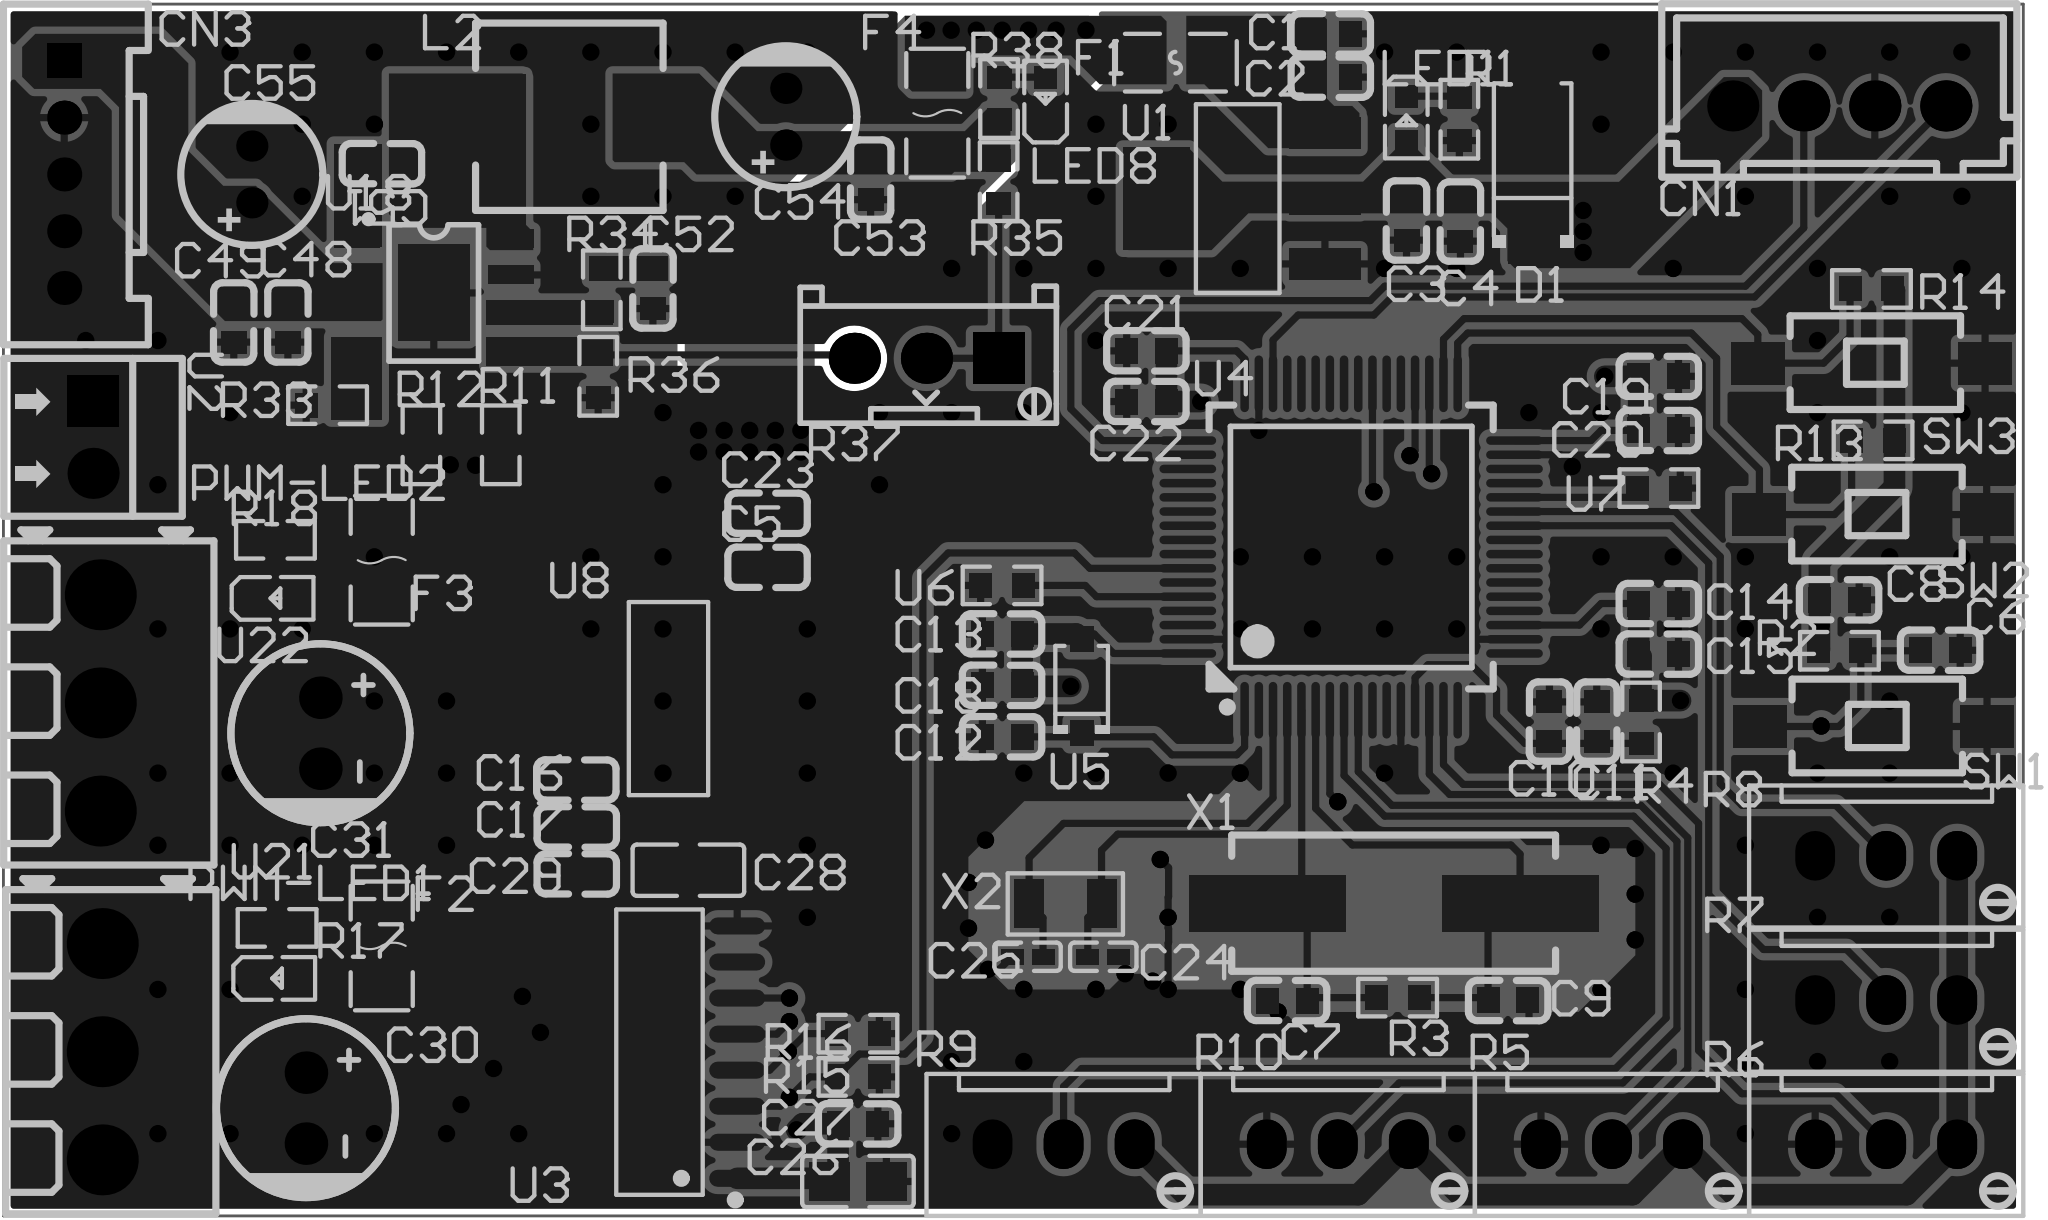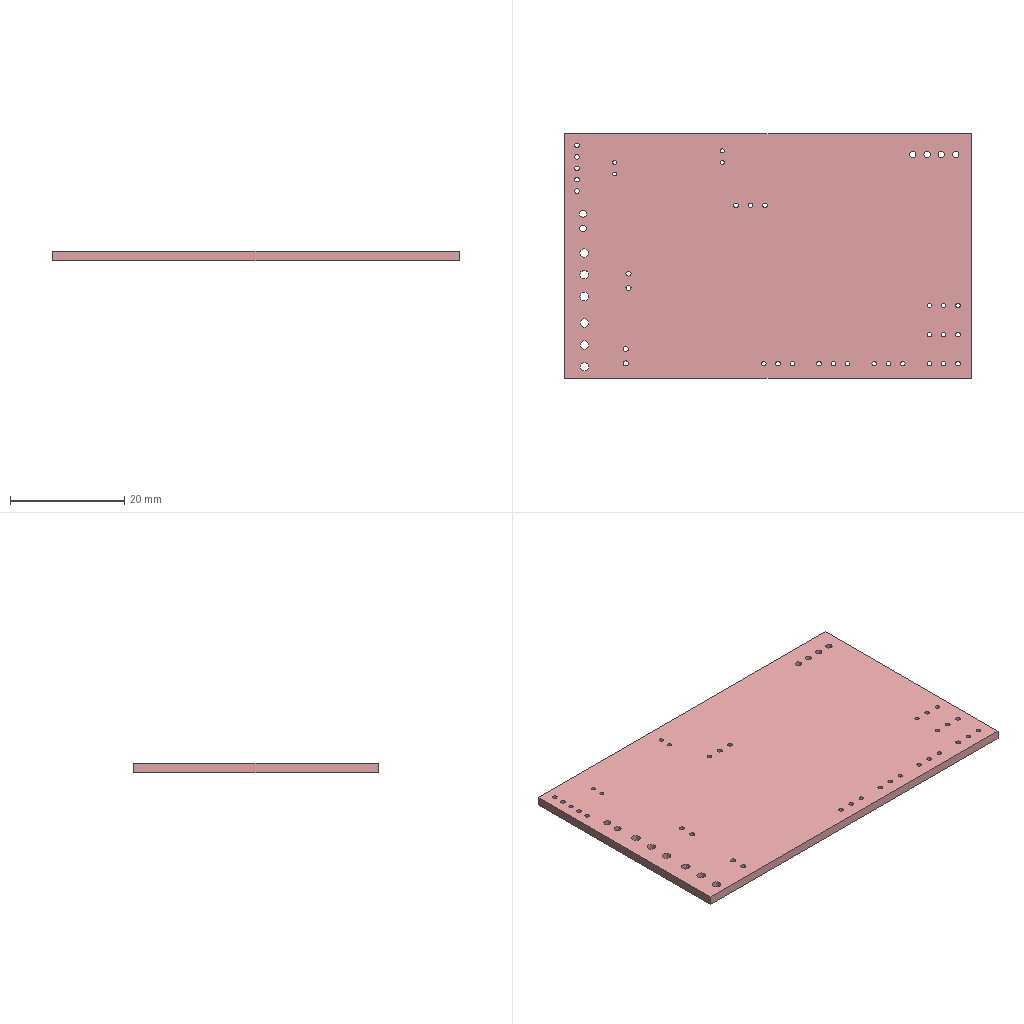Circuit board layout | Altium Designer | box 71.1 x 42.7 x 1.6 mm
Layer stack:
# Altium Designer layer stack of  (unit mm; dielectric type: 0 none, 1 core, 2 prepreg, 3 surface material)
index,name,kind,layer,copper_thickness_mm,dielectric_type,dielectric_thickness_mm,dielectric_material,dielectric_constant
0,Top Paste Mask Layer,other,,,,,,
1,Top Silkscreen Layer,other,,,,,,
2,Top Solder Mask Layer,dielectric,,,3,0.01,,3.3
3,Top Layer,copper,Top Layer,0.035,,,,
4,Dielectric1,dielectric,,,3,1.51,FR4,4.5
5,Bottom Layer,copper,Bottom Layer,0.035,,,,
6,Bottom Solder Mask Layer,dielectric,,,3,0.01,,3.3
7,Bottom Silkscreen Layer,other,,,,,,
8,Bottom Paste Mask Layer,other,,,,,,
# drill layer pairs: low layer,high layer
drill_pair,Top Layer,Bottom Layer
Part placement:
Designator,Comment,Layer,Footprint,Center-X(mm),Center-Y(mm),Rotation
C1,22uF,TopLayer,C0603,125.476,120.777,180
C2,100nF,TopLayer,C0603,125.476,119.253,180
C3,22uF,TopLayer,C0603,128.149,114.209,90
C4,100nF,TopLayer,C0603,130.048,114.173,90
C5,100nF,TopLayer,C0603,105.664,101.981,0
C6,100nF,TopLayer,C0603,146.939,99.06,0
C7,20pF,TopLayer,C0603,123.952,86.719,0
C8,100nF,TopLayer,C0603,143.383,100.838,0
C9,20pF,TopLayer,C0603,131.719,86.724,180
C10,100nF,TopLayer,C0603,133.179,96.542,270
C11,22uF,TopLayer,C0603,134.845,96.542,270
C12,100nF,TopLayer,C0603,113.919,96.012,0
C13,100nF,TopLayer,C0603,113.919,99.635,0
C14,100nF,TopLayer,C0603,137.022,100.708,180
C15,100nF,TopLayer,C0603,137.022,98.93,180
C16,22uF,TopLayer,C0603,98.933,94.488,0
C17,100nF,TopLayer,C0603,98.948,92.834,0
C18,100nF,TopLayer,C0603,113.919,97.823,0
C19,100nF,TopLayer,C0603,137.022,108.712,180
C20,100nF,TopLayer,C0603,137.022,106.807,180
C21,100nF,TopLayer,C0603,118.999,109.608,0
C22,100nF,TopLayer,C0603,118.999,107.824,0
C23,22uF,TopLayer,C0603,105.664,103.886,0
C24,9pF,TopLayer,C0402,117.475,88.265,180
C25,9pF,TopLayer,C0402,114.808,88.265,0
C26,10uF,TopLayer,C0805,108.839,80.349,0
C27,100nF,TopLayer,C0603,108.839,82.381,180
C28,10uF,TopLayer,C0805,102.87,91.313,180
C29,100nF,TopLayer,C0603,98.933,91.186,180
C30,1000uF,TopLayer,CAP-TH_BD6.3-P2.50-D0.5-FD,89.408,82.931,270
C31,1000uF,TopLayer,CAP-TH_BD6.3-P2.50-D0.5-FD,89.916,96.139,270
C48,100nF,TopLayer,C0603,88.773,110.617,90
C49,4.7uF,TopLayer,C0603,86.868,110.617,90
C51,100nF,TopLayer,C0603,92.075,116.205,180
C52,4.7nF,TopLayer,C0603,101.621,111.799,270
C53,47uF,TopLayer,C0603,109.285,115.635,270
C54,100uF,TopLayer,CAP-TH_BD5.0-P2.00-D0.5-FD,106.299,117.856,90
C55,100uF,TopLayer,CAP-TH_BD5.0-P2.00-D0.5-FD,87.503,115.824,90
CN1,HX25003-4A,TopLayer,CONN-TH_4P-P2.50_HX25003-4A,143.383,118.237,180
CN3,ZX-HY2.0-5PZZ,TopLayer,CONN-TH_5P-P2.00_ZX-HY2.0-5PZZ,80.899,115.824,90
D1,SS14,TopLayer,SMA_L4.2-W2.6-LS5.3-RD,132.588,116.332,90
F1,PICOSMDC050S-2,TopLayer,F0805,120.015,119.761,0
F2,JK-nSMD050-30,TopLayer,F1206,92.075,88.646,90
F3,JK-nSMD050-30,TopLayer,F1206,92.075,102.235,90
F4,SMD1206-050-16,TopLayer,F1206,111.633,117.983,90
L2,4.7uH,TopLayer,0630_TPC_7*7*3,98.679,117.856,0
LED1,,TopLayer,LED_0603,128.135,117.78,270
LED8,,TopLayer,LED_0603,115.451,118.44,90
PWM-LED1,,TopLayer,LED_0603,88.341,87.495,0
PWM-LED2,,TopLayer,LED_0603,88.283,100.884,0
R1,1kΩ,TopLayer,R0603,130.009,117.77,90
R2,10kΩ,TopLayer,R0603,143.387,99.044,0
R3,1MΩ,TopLayer,R0603,127.835,86.824,0
R4,10Ω,TopLayer,R0603,136.405,96.534,270
R5,5kΩ,TopLayer,RES-ADJ-TH_3296W-1-203,135.382,81.661,0
R6,5kΩ,TopLayer,RES-ADJ-TH_3296W-1-203,145.034,81.661,0
R7,5kΩ,TopLayer,RES-ADJ-TH_3296W-1-203,145.034,86.741,0
R8,5kΩ,TopLayer,RES-ADJ-TH_3296W-1-203,145.034,91.821,0
R9,5kΩ,TopLayer,RES-ADJ-TH_3296W-1-203,116.078,81.661,0
R10,5kΩ,TopLayer,RES-ADJ-TH_3296W-1-203,125.73,81.661,0
R11,10kΩ,TopLayer,R0603,96.266,106.299,270
R12,10kΩ,TopLayer,R0603,93.472,106.299,270
R13,10kΩ,TopLayer,R0603,144.571,106.456,180
R14,10kΩ,TopLayer,R0603,144.515,111.79,180
R15,10kΩ,TopLayer,R0603,108.839,84.032,180
R16,10kΩ,TopLayer,R0603,108.839,85.556,180
R17,1kΩ,TopLayer,R0603,88.392,89.281,180
R18,1kΩ,TopLayer,R0603,88.334,102.953,180
R33,200K,TopLayer,R0603,90.17,107.696,0
R34,20K,TopLayer,R0603,99.822,111.76,90
R35,27k,TopLayer,R0603,113.792,115.57,90
R36,8.2K,TopLayer,R0603,99.695,108.712,90
R37,50K,TopLayer,RESPOT3296,111.252,109.347,180
R38,1k,TopLayer,R0603,113.806,118.498,270
SW1,TS-1101-C-W,TopLayer,SW-SMD_L6.0-W3.3-LS8.0,144.583,96.377,180
SW2,TS-1101-C-W,TopLayer,SW-SMD_L6.0-W3.3-LS8.0,144.571,103.841,180
SW3,TS-1101-C-W,TopLayer,SW-SMD_L6.0-W3.3-LS8.0,144.515,109.175,180
U1,AMS1117-3.3,TopLayer,SOT-223-3_L6.5-W3.4-P2.30-LS7.0-BR,122.307,114.971,0
U2,DB125-2.54-2P-GN-S,TopLayer,CONN-TH_DB125-2.54-2P-GN,81.915,106.563,270
U3,p142U31,TopLayer,SOIC-16_L9.9-W3.9-P1.27-LS6.0-BL,101.853,84.904,90
U4,STM32F103RET6,TopLayer,LQFP-64_L10.0-W10.0-P0.50-LS12.0-BL,126.2,102.698,0
U5,IN4148 SMD diode,TopLayer,SOD-123_L2.7-W1.7-LS3.8-RD,116.713,97.79,90
U6,100k,TopLayer,R0603,113.911,101.346,180
U7,100k,TopLayer,R0603,137.033,104.775,180
U8,AMS1117-5.0,TopLayer,SOT-223_L6.5-W3.5-P2.30-LS7.0-BR,102.17,97.359,0
U18,SCT2450,TopLayer,SOP-8E,93.909,111.648,0
U21,DB125-3.81-3P-GN-S,TopLayer,CONN-TH_3P-P3.81_L7.4-W11.4,82.238,84.919,270
U22,DB125-3.81-3P-GN-S,TopLayer,CONN-TH_3P-P3.81_L7.4-W11.4,82.169,97.206,270
X1,8MHz,TopLayer,CRYSTAL-SMD_L11.5-W4.8-LS12.7,127.696,90.153,0
X2,32.768kHz,TopLayer,OSC-SMD_L3.2-W1.5,116.139,90.126,0
Pad and via stacks:
# Altium Designer via and pad stacks of  (unit mm). Each distinct definition once, with the count of objects using it.
# via: kind,start_layer,end_layer,hole_mm,diameter_mm,mode(0 simple;1 top-mid-bottom;2 full stack),diameter_per_layer,count,example_net
# pad: kind,layer,hole_mm,hole_type(0 round;1 square;2 slot),plating,top_size,top_shape(1 round;2 rect;3 octagon;9 rounded rect),mid_size,bottom_size,mode,footprint,size_per_layer,count,example
pad,Top Layer,0,0,plated,0.8x0.9,2,0.8x0.9,0.8x0.9,0,C0603,,60,C1.2
pad,Top Layer,0,0,plated,0.7901x0.54,2,0.7901x0.54,0.7901x0.54,0,C0402,,4,C24.2
pad,Top Layer,0,0,plated,1.41x1.35,2,1.41x1.35,1.41x1.35,0,C0805,,4,C26.2
pad,Top Layer,0,0,plated,2.2x1.7,2,2.2x1.7,2.2x1.7,0,SMA_L4.2-W2.6-LS5.3-RD,,2,D1.1
pad,Top Layer,0,0,plated,1.335x1.5,2,1.335x1.5,1.335x1.5,0,F0805,,2,F1.2
pad,Top Layer,0,0,plated,1.19x1.728,2,1.19x1.728,1.19x1.728,0,F1206,,6,F2.1
pad,Top Layer,0,0,plated,2.5x3,2,2.5x3,2.5x3,0,0630 TPC 7*7*3,,2,L2.1
pad,Top Layer,0,0,plated,0.8001x0.8001,2,0.8001x0.8001,0.8001x0.8001,0,LED_0603,,8,LED1.1
pad,Top Layer,0,0,plated,0.8065x0.864,2,0.8065x0.864,0.8065x0.864,0,R0603,,38,R1.2
pad,Top Layer,0,0,plated,1.9x1.5,2,1.9x1.5,1.9x1.5,0,SW-SMD_L6.0-W3.3-LS8.0,,6,SW1.1
pad,Top Layer,0,0,plated,2.5x1.1,2,2.5x1.1,2.5x1.1,0,SOT-223-3_L6.5-W3.4-P2.30-LS7.0-BR,,3,U1.1
pad,Top Layer,0,0,plated,2.34x3.6,2,2.34x3.6,2.34x3.6,0,SOT-223-3_L6.5-W3.4-P2.30-LS7.0-BR,,1,U1.4
pad,Top Layer,0,0,plated,0.602x1.971,1,0.602x1.971,0.602x1.971,0,SOIC-16_L9.9-W3.9-P1.27-LS6.0-BL,,16,U3.1
pad,Top Layer,0,0,plated,2x0.3,1,2x0.3,2x0.3,0,LQFP-64_L10.0-W10.0-P0.50-LS12.0-BL,,32,U4.64
pad,Top Layer,0,0,plated,0.3x2,1,0.3x2,0.3x2,0,LQFP-64_L10.0-W10.0-P0.50-LS12.0-BL,,32,U4.48
pad,Top Layer,0,0,plated,0.91x0.84,2,0.91x0.84,0.91x0.84,0,SOD-123_L2.7-W1.7-LS3.8-RD,,2,U5.1
pad,Top Layer,0,0,plated,2.465x1.05,2,2.465x1.05,2.465x1.05,0,SOT-223_L6.5-W3.5-P2.30-LS7.0-BR,,3,U8.1
pad,Top Layer,0,0,plated,2.465x3.54,2,2.465x3.54,2.465x3.54,0,SOT-223_L6.5-W3.5-P2.30-LS7.0-BR,,1,U8.4
pad,Top Layer,0,0,unplated,1.6x0.65,2,1.6x0.65,1.6x0.65,0,SOP-8E,,8,U18.8
pad,Top Layer,0,0,unplated,2.5x3.4,2,2.5x3.4,2.5x3.4,0,SOP-8E,,1,U18.0
pad,Top Layer,0,0,plated,5.5x2,2,5.5x2,5.5x2,0,CRYSTAL-SMD_L11.5-W4.8-LS12.7,,2,X1.2
pad,Top Layer,0,0,plated,1.05x1.7,2,1.05x1.7,1.05x1.7,0,OSC-SMD_L3.2-W1.5,,2,X2.1
pad,Multi-Layer,0.9,0,plated,1.5x1.5,1,1.5x1.5,1.5x1.5,0,CAP-TH_BD6.3-P2.50-D0.5-FD,,4,C30.2
pad,Multi-Layer,0.7,0,plated,1.1x1.1,1,1.1x1.1,1.1x1.1,0,CAP-TH_BD5.0-P2.00-D0.5-FD,,4,C54.1
pad,Multi-Layer,1.1,0,plated,1.8x1.8,1,1.8x1.8,1.8x1.8,0,CONN-TH_4P-P2.50_HX25003-4A,,4,CN1.1
pad,Multi-Layer,0.8,0,plated,1.2x1.2,1,1.2x1.2,1.2x1.2,0,CONN-TH_5P-P2.00_ZX-HY2.0-5PZZ,,4,CN3.5
pad,Multi-Layer,0.8,0,plated,1.2x1.2,2,1.2x1.2,1.2x1.2,0,CONN-TH_5P-P2.00_ZX-HY2.0-5PZZ,,1,CN3.1
pad,Multi-Layer,0.8,0,plated,1.4x1.75,1,1.4x1.75,1.4x1.75,0,RES-ADJ-TH_3296W-1-203,,18,R5.1
pad,Multi-Layer,0.8,0,plated,1.8x1.8,1,1.8x1.8,1.8x1.8,0,RESPOT3296,,2,R37.2
pad,Multi-Layer,0.8,0,plated,1.8x1.8,2,1.8x1.8,1.8x1.8,0,RESPOT3296,,1,R37.1
pad,Multi-Layer,1.2,0,plated,1.8x1.8,1,1.8x1.8,1.8x1.8,0,CONN-TH_DB125-2.54-2P-GN,,1,U2.2
pad,Multi-Layer,1.2,0,plated,1.8x1.8,2,1.8x1.8,1.8x1.8,0,CONN-TH_DB125-2.54-2P-GN,,1,U2.1
pad,Multi-Layer,1.5,0,plated,2.5x2.5,1,2.5x2.5,2.5x2.5,0,CONN-TH_3P-P3.81_L7.4-W11.4,,6,U21.1
via,Top Layer,Bottom Layer,0.3048,0.61,0,,188,NRST
Copper pours:
name,layer,net,type(0 solid;1 hatched;2 none)
Top Layer-GND,Top Layer,GND,0
Bottom Layer-GND,Bottom Layer,GND,0